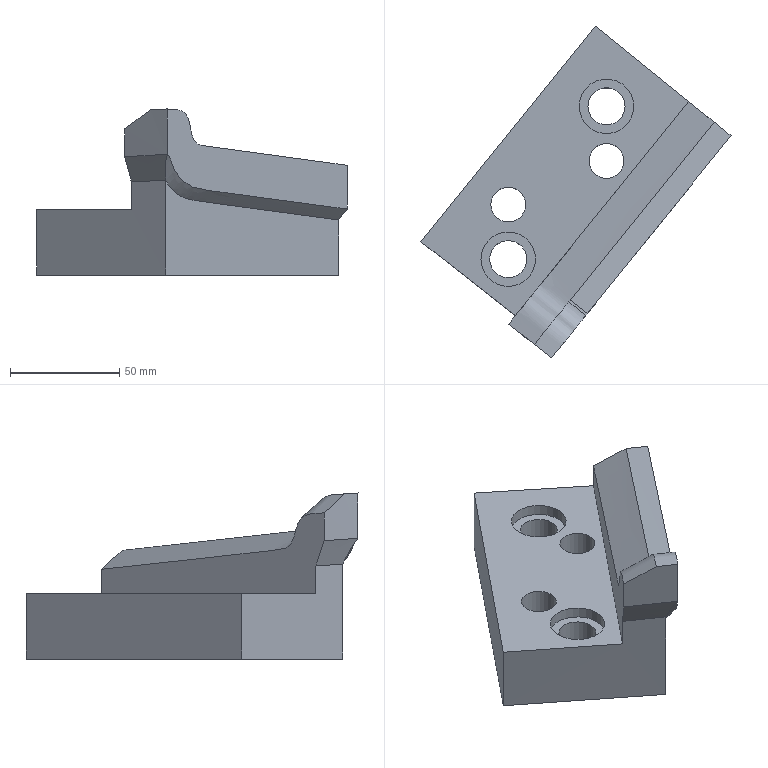Part | NX | features solid 2 | 1 solid | 23 faces | box 142.057 x 152.073 x 76.099 mm | volume 333815 mm3 | plane 9 | spline 8 | cylinder 6 | commonest cylinder face diameters 16 x2 17 x2 25 x2